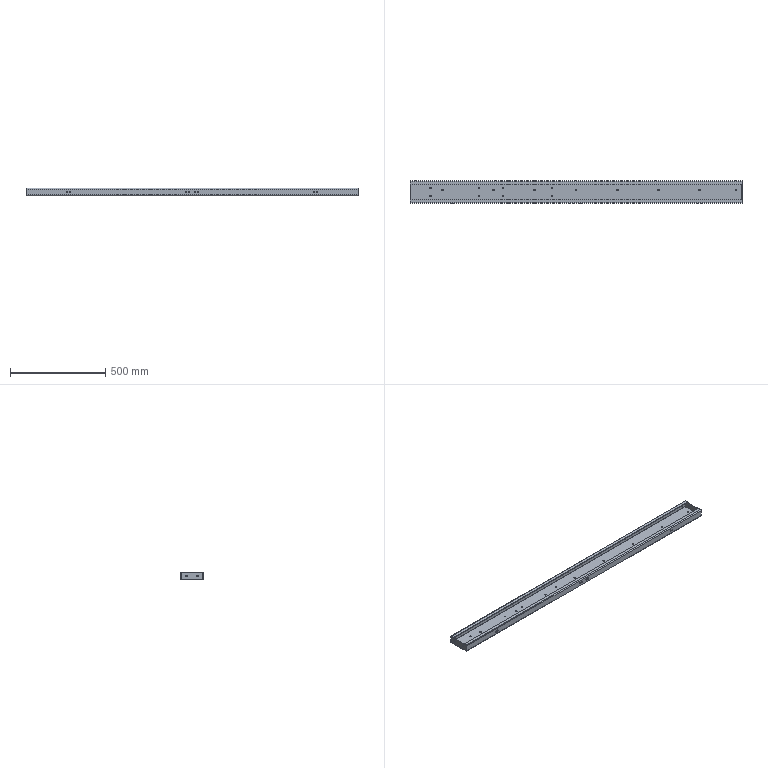Part | SolidWorks | features BaseBody 3 | 3 solids | 124 faces | box 1740 x 120 x 40 mm | volume 1547696 mm3 | cylinder 66 | plane 58 | commonest cylinder face diameters 7 x16 8.5 x16 9 x16 5 x10 1.473 x4 9.473 x4